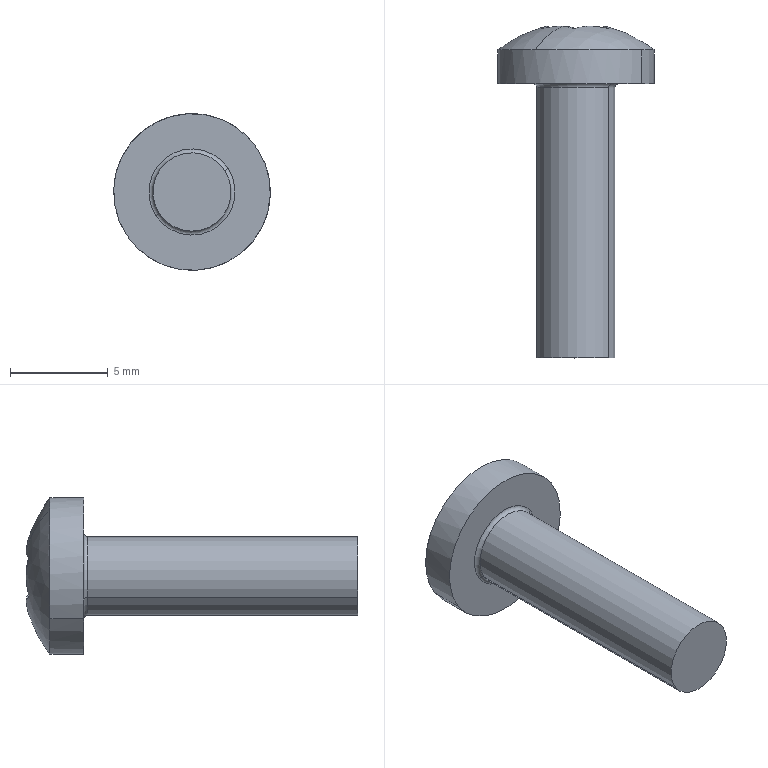Part | SolidWorks | features BaseBody 1 | 1 solid | 23 faces | box 8 x 16.943 x 8 mm | volume 285.559 mm3 | plane 15 | cylinder 4 | sphere 2 | torus 2 | commonest cylinder face diameters 4 x2 8 x2
STEP:
#1=CARTESIAN_POINT('',(202.131,119.073,289.752));
#2=VERTEX_POINT('',#1);
#3=CARTESIAN_POINT('',(203.395,119.073,295.353));
#4=VERTEX_POINT('',#3);
#5=CARTESIAN_POINT('',(205.48,119.073,291.94));
#6=DIRECTION('',(0.,1.,0.));
#7=DIRECTION('',(0.8372,0.,0.5469));
#8=AXIS2_PLACEMENT_3D('',#5,#6,#7);
#9=CIRCLE('',#8,4.);
#10=EDGE_CURVE('',#2,#4,#9,.T.);
#11=ORIENTED_EDGE('',*,*,#10,.T.);
#12=CARTESIAN_POINT('',(204.804,120.281,293.249));
#13=VERTEX_POINT('',#12);
#14=CARTESIAN_POINT('',(205.48,113.95,291.94));
#15=DIRECTION('',(-0.8369,0.02365,-0.5468));
#16=DIRECTION('',(-0.5469,0.,0.8372));
#17=AXIS2_PLACEMENT_3D('',#14,#15,#16);
#18=CIRCLE('',#17,6.5);
#19=EDGE_CURVE('',#4,#13,#18,.T.);
#20=ORIENTED_EDGE('',*,*,#19,.T.);
#21=CARTESIAN_POINT('',(204.702,120.293,293.13));
#22=VERTEX_POINT('',#21);
#23=CARTESIAN_POINT('',(204.443,113.95,292.828));
#24=DIRECTION('',(-0.7597,0.,0.6503));
#25=DIRECTION('',(0.1461,0.9744,0.1706));
#26=AXIS2_PLACEMENT_3D('',#23,#24,#25);
#27=CIRCLE('',#26,6.355);
#28=EDGE_CURVE('',#13,#22,#27,.T.);
#29=ORIENTED_EDGE('',*,*,#28,.T.);
#30=CARTESIAN_POINT('',(203.718,120.143,292.832));
#31=VERTEX_POINT('',#30);
#32=CARTESIAN_POINT('',(205.084,113.95,293.246));
#33=DIRECTION('',(-0.2903,0.,0.9569));
#34=DIRECTION('',(-0.06003,0.998,-0.01821));
#35=AXIS2_PLACEMENT_3D('',#32,#33,#34);
#36=CIRCLE('',#35,6.355);
#37=EDGE_CURVE('',#22,#31,#36,.T.);
#38=ORIENTED_EDGE('',*,*,#37,.T.);
#39=CARTESIAN_POINT('',(204.06,120.293,291.862));
#40=VERTEX_POINT('',#39);
#41=CARTESIAN_POINT('',(204.193,113.95,291.486));
#42=DIRECTION('',(-0.943,0.,-0.3328));
#43=DIRECTION('',(-0.07475,0.9744,0.2118));
#44=AXIS2_PLACEMENT_3D('',#41,#42,#43);
#45=CIRCLE('',#44,6.355);
#46=EDGE_CURVE('',#31,#40,#45,.T.);
#47=ORIENTED_EDGE('',*,*,#46,.T.);
#48=CARTESIAN_POINT('',(203.827,120.143,290.86));
#49=VERTEX_POINT('',#48);
#50=CARTESIAN_POINT('',(204.151,113.95,292.25));
#51=DIRECTION('',(-0.9739,0.,0.227));
#52=DIRECTION('',(-0.01424,0.998,-0.06109));
#53=AXIS2_PLACEMENT_3D('',#50,#51,#52);
#54=CIRCLE('',#53,6.355);
#55=EDGE_CURVE('',#40,#49,#54,.T.);
#56=ORIENTED_EDGE('',*,*,#55,.T.);
#57=CARTESIAN_POINT('',(204.838,120.293,290.671));
#58=VERTEX_POINT('',#57);
#59=CARTESIAN_POINT('',(205.23,113.95,290.598));
#60=DIRECTION('',(-0.1833,0.,-0.9831));
#61=DIRECTION('',(-0.2208,0.9744,0.04117));
#62=AXIS2_PLACEMENT_3D('',#59,#60,#61);
#63=CIRCLE('',#62,6.355);
#64=EDGE_CURVE('',#49,#58,#63,.T.);
#65=ORIENTED_EDGE('',*,*,#64,.T.);
#66=CARTESIAN_POINT('',(205.589,120.143,289.968));
#67=VERTEX_POINT('',#66);
#68=CARTESIAN_POINT('',(204.547,113.95,290.944));
#69=DIRECTION('',(-0.6836,0.,-0.7299));
#70=DIRECTION('',(0.04578,0.998,-0.04288));
#71=AXIS2_PLACEMENT_3D('',#68,#69,#70);
#72=CIRCLE('',#71,6.355);
#73=EDGE_CURVE('',#58,#67,#72,.T.);
#74=ORIENTED_EDGE('',*,*,#73,.T.);
#75=CARTESIAN_POINT('',(206.258,120.293,290.75));
#76=VERTEX_POINT('',#75);
#77=CARTESIAN_POINT('',(206.517,113.95,291.052));
#78=DIRECTION('',(0.7597,0.,-0.6503));
#79=DIRECTION('',(-0.1461,0.9744,-0.1706));
#80=AXIS2_PLACEMENT_3D('',#77,#78,#79);
#81=CIRCLE('',#80,6.355);
#82=EDGE_CURVE('',#67,#76,#81,.T.);
#83=ORIENTED_EDGE('',*,*,#82,.T.);
#84=CARTESIAN_POINT('',(206.407,120.281,290.795));
#85=VERTEX_POINT('',#84);
#86=CARTESIAN_POINT('',(205.876,113.95,290.634));
#87=DIRECTION('',(0.2903,0.,-0.9569));
#88=DIRECTION('',(0.06003,0.998,0.01821));
#89=AXIS2_PLACEMENT_3D('',#86,#87,#88);
#90=CIRCLE('',#89,6.355);
#91=EDGE_CURVE('',#76,#85,#90,.T.);
#92=ORIENTED_EDGE('',*,*,#91,.T.);
#93=CARTESIAN_POINT('',(207.768,119.073,288.659));
#94=VERTEX_POINT('',#93);
#95=CARTESIAN_POINT('',(205.48,113.95,291.94));
#96=DIRECTION('',(-0.8369,0.02365,-0.5468));
#97=DIRECTION('',(-0.5469,0.,0.8372));
#98=AXIS2_PLACEMENT_3D('',#95,#96,#97);
#99=CIRCLE('',#98,6.5);
#100=EDGE_CURVE('',#85,#94,#99,.T.);
#101=ORIENTED_EDGE('',*,*,#100,.T.);
#102=CARTESIAN_POINT('',(205.48,119.073,291.94));
#103=DIRECTION('',(0.,1.,0.));
#104=DIRECTION('',(0.8372,0.,0.5469));
#105=AXIS2_PLACEMENT_3D('',#102,#103,#104);
#106=CIRCLE('',#105,4.);
#107=EDGE_CURVE('',#94,#2,#106,.T.);
#108=ORIENTED_EDGE('',*,*,#107,.T.);
#109=EDGE_LOOP('',(#11,#20,#29,#38,#47,#56,#65,#74,#83,#92,#101,#108));
#110=FACE_OUTER_BOUND('',#109,.T.);
#111=CARTESIAN_POINT('',(205.48,113.95,291.94));
#112=DIRECTION('',(0.8369,-0.02365,0.5468));
#113=DIRECTION('',(0.0198,0.9997,0.01294));
#114=AXIS2_PLACEMENT_3D('',#111,#112,#113);
#115=SPHERICAL_SURFACE('',#114,6.5);
#116=ADVANCED_FACE('',(#110),#115,.T.);
#117=CARTESIAN_POINT('',(202.131,117.35,289.752));
#118=VERTEX_POINT('',#117);
#119=CARTESIAN_POINT('',(208.829,117.35,294.128));
#120=VERTEX_POINT('',#119);
#121=CARTESIAN_POINT('',(205.48,117.35,291.94));
#122=DIRECTION('',(0.,1.,0.));
#123=DIRECTION('',(0.8372,0.,0.5469));
#124=AXIS2_PLACEMENT_3D('',#121,#122,#123);
#125=CIRCLE('',#124,4.);
#126=EDGE_CURVE('',#118,#120,#125,.T.);
#127=ORIENTED_EDGE('',*,*,#126,.T.);
#128=CARTESIAN_POINT('',(208.829,119.073,294.128));
#129=VERTEX_POINT('',#128);
#130=CARTESIAN_POINT('',(208.829,117.35,294.128));
#131=DIRECTION('',(0.,1.,0.));
#132=VECTOR('',#131,1000.);
#133=LINE('',#130,#132);
#134=EDGE_CURVE('',#120,#129,#133,.T.);
#135=ORIENTED_EDGE('',*,*,#134,.T.);
#136=CARTESIAN_POINT('',(205.48,119.073,291.94));
#137=DIRECTION('',(0.,1.,0.));
#138=DIRECTION('',(0.8372,0.,0.5469));
#139=AXIS2_PLACEMENT_3D('',#136,#137,#138);
#140=CIRCLE('',#139,4.);
#141=EDGE_CURVE('',#4,#129,#140,.T.);
#142=ORIENTED_EDGE('',*,*,#141,.F.);
#143=ORIENTED_EDGE('',*,*,#10,.F.);
#144=CARTESIAN_POINT('',(202.131,117.35,289.752));
#145=DIRECTION('',(0.,1.,0.));
#146=VECTOR('',#145,1000.);
#147=LINE('',#144,#146);
#148=EDGE_CURVE('',#118,#2,#147,.T.);
#149=ORIENTED_EDGE('',*,*,#148,.F.);
#150=EDGE_LOOP('',(#127,#135,#142,#143,#149));
#151=FACE_OUTER_BOUND('',#150,.T.);
#152=CARTESIAN_POINT('',(205.48,117.35,291.94));
#153=DIRECTION('',(0.,1.,0.));
#154=DIRECTION('',(-0.8372,0.,-0.5469));
#155=AXIS2_PLACEMENT_3D('',#152,#153,#154);
#156=CYLINDRICAL_SURFACE('',#155,4.);
#157=ADVANCED_FACE('',(#151),#156,.T.);
#158=CARTESIAN_POINT('',(207.154,103.35,293.034));
#159=VERTEX_POINT('',#158);
#160=CARTESIAN_POINT('',(203.806,103.35,290.846));
#161=VERTEX_POINT('',#160);
#162=CARTESIAN_POINT('',(205.48,103.35,291.94));
#163=DIRECTION('',(0.,-1.,0.));
#164=DIRECTION('',(0.8372,0.,0.5469));
#165=AXIS2_PLACEMENT_3D('',#162,#163,#164);
#166=CIRCLE('',#165,2.);
#167=EDGE_CURVE('',#159,#161,#166,.T.);
#168=ORIENTED_EDGE('',*,*,#167,.F.);
#169=CARTESIAN_POINT('',(207.154,117.15,293.034));
#170=VERTEX_POINT('',#169);
#171=CARTESIAN_POINT('',(207.154,103.35,293.034));
#172=DIRECTION('',(0.,1.,0.));
#173=VECTOR('',#172,1000.);
#174=LINE('',#171,#173);
#175=EDGE_CURVE('',#159,#170,#174,.T.);
#176=ORIENTED_EDGE('',*,*,#175,.T.);
#177=CARTESIAN_POINT('',(203.806,117.15,290.846));
#178=VERTEX_POINT('',#177);
#179=CARTESIAN_POINT('',(205.48,117.15,291.94));
#180=DIRECTION('',(0.,-1.,0.));
#181=DIRECTION('',(0.8372,0.,0.5469));
#182=AXIS2_PLACEMENT_3D('',#179,#180,#181);
#183=CIRCLE('',#182,2.);
#184=EDGE_CURVE('',#170,#178,#183,.T.);
#185=ORIENTED_EDGE('',*,*,#184,.T.);
#186=CARTESIAN_POINT('',(203.806,103.35,290.846));
#187=DIRECTION('',(0.,1.,0.));
#188=VECTOR('',#187,1000.);
#189=LINE('',#186,#188);
#190=EDGE_CURVE('',#161,#178,#189,.T.);
#191=ORIENTED_EDGE('',*,*,#190,.F.);
#192=EDGE_LOOP('',(#168,#176,#185,#191));
#193=FACE_OUTER_BOUND('',#192,.T.);
#194=CARTESIAN_POINT('',(205.48,103.35,291.94));
#195=DIRECTION('',(0.,1.,0.));
#196=DIRECTION('',(-0.8372,0.,-0.5469));
#197=AXIS2_PLACEMENT_3D('',#194,#195,#196);
#198=CYLINDRICAL_SURFACE('',#197,2.);
#199=ADVANCED_FACE('',(#193),#198,.T.);
#200=CARTESIAN_POINT('',(207.322,117.35,293.143));
#201=VERTEX_POINT('',#200);
#202=CARTESIAN_POINT('',(203.638,117.35,290.737));
#203=VERTEX_POINT('',#202);
#204=CARTESIAN_POINT('',(205.48,117.35,291.94));
#205=DIRECTION('',(0.,1.,0.));
#206=DIRECTION('',(0.8372,0.,0.5469));
#207=AXIS2_PLACEMENT_3D('',#204,#205,#206);
#208=CIRCLE('',#207,2.2);
#209=EDGE_CURVE('',#201,#203,#208,.T.);
#210=ORIENTED_EDGE('',*,*,#209,.F.);
#211=CARTESIAN_POINT('',(207.322,117.15,293.143));
#212=DIRECTION('',(-0.5469,0.,0.8372));
#213=DIRECTION('',(0.8372,0.,0.5469));
#214=AXIS2_PLACEMENT_3D('',#211,#212,#213);
#215=CIRCLE('',#214,0.2);
#216=EDGE_CURVE('',#201,#170,#215,.T.);
#217=ORIENTED_EDGE('',*,*,#216,.T.);
#218=CARTESIAN_POINT('',(205.48,117.15,291.94));
#219=DIRECTION('',(0.,-1.,0.));
#220=DIRECTION('',(0.8372,0.,0.5469));
#221=AXIS2_PLACEMENT_3D('',#218,#219,#220);
#222=CIRCLE('',#221,2.);
#223=EDGE_CURVE('',#178,#170,#222,.T.);
#224=ORIENTED_EDGE('',*,*,#223,.F.);
#225=CARTESIAN_POINT('',(203.638,117.15,290.737));
#226=DIRECTION('',(0.5469,0.,-0.8372));
#227=DIRECTION('',(-0.8372,0.,-0.5469));
#228=AXIS2_PLACEMENT_3D('',#225,#226,#227);
#229=CIRCLE('',#228,0.2);
#230=EDGE_CURVE('',#203,#178,#229,.T.);
#231=ORIENTED_EDGE('',*,*,#230,.F.);
#232=EDGE_LOOP('',(#210,#217,#224,#231));
#233=FACE_OUTER_BOUND('',#232,.T.);
#234=CARTESIAN_POINT('',(205.48,117.15,291.94));
#235=DIRECTION('',(0.,1.,0.));
#236=DIRECTION('',(-0.8372,0.,-0.5469));
#237=AXIS2_PLACEMENT_3D('',#234,#235,#236);
#238=TOROIDAL_SURFACE('',#237,2.2,0.2);
#239=ADVANCED_FACE('',(#233),#238,.F.);
#240=CARTESIAN_POINT('',(206.9,118.79,292.018));
#241=VERTEX_POINT('',#240);
#242=CARTESIAN_POINT('',(207.133,118.79,293.02));
#243=VERTEX_POINT('',#242);
#244=CARTESIAN_POINT('',(206.9,118.79,292.018));
#245=DIRECTION('',(0.227,0.,0.9739));
#246=VECTOR('',#245,1000.);
#247=LINE('',#244,#246);
#248=EDGE_CURVE('',#241,#243,#247,.T.);
#249=ORIENTED_EDGE('',*,*,#248,.F.);
#250=CARTESIAN_POINT('',(207.242,118.79,291.048));
#251=VERTEX_POINT('',#250);
#252=CARTESIAN_POINT('',(207.242,118.79,291.048));
#253=DIRECTION('',(-0.3328,0.,0.943));
#254=VECTOR('',#253,1000.);
#255=LINE('',#252,#254);
#256=EDGE_CURVE('',#251,#241,#255,.T.);
#257=ORIENTED_EDGE('',*,*,#256,.F.);
#258=CARTESIAN_POINT('',(206.258,118.79,290.75));
#259=VERTEX_POINT('',#258);
#260=CARTESIAN_POINT('',(206.258,118.79,290.75));
#261=DIRECTION('',(0.9569,0.,0.2903));
#262=VECTOR('',#261,1000.);
#263=LINE('',#260,#262);
#264=EDGE_CURVE('',#259,#251,#263,.T.);
#265=ORIENTED_EDGE('',*,*,#264,.F.);
#266=CARTESIAN_POINT('',(205.589,118.79,289.968));
#267=VERTEX_POINT('',#266);
#268=CARTESIAN_POINT('',(205.589,118.79,289.968));
#269=DIRECTION('',(0.6503,0.,0.7597));
#270=VECTOR('',#269,1000.);
#271=LINE('',#268,#270);
#272=EDGE_CURVE('',#267,#259,#271,.T.);
#273=ORIENTED_EDGE('',*,*,#272,.F.);
#274=CARTESIAN_POINT('',(204.838,118.79,290.671));
#275=VERTEX_POINT('',#274);
#276=CARTESIAN_POINT('',(204.838,118.79,290.671));
#277=DIRECTION('',(0.7299,0.,-0.6836));
#278=VECTOR('',#277,1000.);
#279=LINE('',#276,#278);
#280=EDGE_CURVE('',#275,#267,#279,.T.);
#281=ORIENTED_EDGE('',*,*,#280,.F.);
#282=CARTESIAN_POINT('',(203.827,118.79,290.86));
#283=VERTEX_POINT('',#282);
#284=CARTESIAN_POINT('',(203.827,118.79,290.86));
#285=DIRECTION('',(0.9831,0.,-0.1833));
#286=VECTOR('',#285,1000.);
#287=LINE('',#284,#286);
#288=EDGE_CURVE('',#283,#275,#287,.T.);
#289=ORIENTED_EDGE('',*,*,#288,.F.);
#290=CARTESIAN_POINT('',(204.06,118.79,291.862));
#291=VERTEX_POINT('',#290);
#292=CARTESIAN_POINT('',(204.06,118.79,291.862));
#293=DIRECTION('',(-0.227,0.,-0.9739));
#294=VECTOR('',#293,1000.);
#295=LINE('',#292,#294);
#296=EDGE_CURVE('',#291,#283,#295,.T.);
#297=ORIENTED_EDGE('',*,*,#296,.F.);
#298=CARTESIAN_POINT('',(203.718,118.79,292.832));
#299=VERTEX_POINT('',#298);
#300=CARTESIAN_POINT('',(203.718,118.79,292.832));
#301=DIRECTION('',(0.3328,0.,-0.943));
#302=VECTOR('',#301,1000.);
#303=LINE('',#300,#302);
#304=EDGE_CURVE('',#299,#291,#303,.T.);
#305=ORIENTED_EDGE('',*,*,#304,.F.);
#306=CARTESIAN_POINT('',(204.702,118.79,293.13));
#307=VERTEX_POINT('',#306);
#308=CARTESIAN_POINT('',(204.702,118.79,293.13));
#309=DIRECTION('',(-0.9569,0.,-0.2903));
#310=VECTOR('',#309,1000.);
#311=LINE('',#308,#310);
#312=EDGE_CURVE('',#307,#299,#311,.T.);
#313=ORIENTED_EDGE('',*,*,#312,.F.);
#314=CARTESIAN_POINT('',(205.371,118.79,293.912));
#315=VERTEX_POINT('',#314);
#316=CARTESIAN_POINT('',(205.371,118.79,293.912));
#317=DIRECTION('',(-0.6503,0.,-0.7597));
#318=VECTOR('',#317,1000.);
#319=LINE('',#316,#318);
#320=EDGE_CURVE('',#315,#307,#319,.T.);
#321=ORIENTED_EDGE('',*,*,#320,.F.);
#322=CARTESIAN_POINT('',(206.122,118.79,293.209));
#323=VERTEX_POINT('',#322);
#324=CARTESIAN_POINT('',(206.122,118.79,293.209));
#325=DIRECTION('',(-0.7299,0.,0.6836));
#326=VECTOR('',#325,1000.);
#327=LINE('',#324,#326);
#328=EDGE_CURVE('',#323,#315,#327,.T.);
#329=ORIENTED_EDGE('',*,*,#328,.F.);
#330=CARTESIAN_POINT('',(207.133,118.79,293.02));
#331=DIRECTION('',(-0.9831,0.,0.1833));
#332=VECTOR('',#331,1000.);
#333=LINE('',#330,#332);
#334=EDGE_CURVE('',#243,#323,#333,.T.);
#335=ORIENTED_EDGE('',*,*,#334,.F.);
#336=EDGE_LOOP('',(#249,#257,#265,#273,#281,#289,#297,#305,#313,#321,#329,#335));
#337=FACE_OUTER_BOUND('',#336,.T.);
#338=CARTESIAN_POINT('',(206.513,118.79,290.359));
#339=DIRECTION('',(0.,1.,0.));
#340=DIRECTION('',(1.,0.,0.));
#341=AXIS2_PLACEMENT_3D('',#338,#339,#340);
#342=PLANE('',#341);
#343=ADVANCED_FACE('',(#337),#342,.T.);
#344=CARTESIAN_POINT('',(207.133,120.143,293.02));
#345=VERTEX_POINT('',#344);
#346=CARTESIAN_POINT('',(207.133,118.79,293.02));
#347=DIRECTION('',(0.,1.,0.));
#348=VECTOR('',#347,1000.);
#349=LINE('',#346,#348);
#350=EDGE_CURVE('',#243,#345,#349,.T.);
#351=ORIENTED_EDGE('',*,*,#350,.F.);
#352=ORIENTED_EDGE('',*,*,#334,.T.);
#353=CARTESIAN_POINT('',(206.122,120.293,293.209));
#354=VERTEX_POINT('',#353);
#355=CARTESIAN_POINT('',(206.122,120.293,293.209));
#356=DIRECTION('',(0.,-1.,0.));
#357=VECTOR('',#356,1000.);
#358=LINE('',#355,#357);
#359=EDGE_CURVE('',#354,#323,#358,.T.);
#360=ORIENTED_EDGE('',*,*,#359,.F.);
#361=CARTESIAN_POINT('',(205.73,113.95,293.282));
#362=DIRECTION('',(0.1833,0.,0.9831));
#363=DIRECTION('',(0.2208,0.9744,-0.04117));
#364=AXIS2_PLACEMENT_3D('',#361,#362,#363);
#365=CIRCLE('',#364,6.355);
#366=EDGE_CURVE('',#345,#354,#365,.T.);
#367=ORIENTED_EDGE('',*,*,#366,.F.);
#368=EDGE_LOOP('',(#351,#352,#360,#367));
#369=FACE_OUTER_BOUND('',#368,.T.);
#370=CARTESIAN_POINT('',(206.122,118.79,293.209));
#371=DIRECTION('',(-0.1833,0.,-0.9831));
#372=DIRECTION('',(-0.9831,0.,0.1833));
#373=AXIS2_PLACEMENT_3D('',#370,#371,#372);
#374=PLANE('',#373);
#375=ADVANCED_FACE('',(#369),#374,.T.);
#376=ORIENTED_EDGE('',*,*,#359,.T.);
#377=ORIENTED_EDGE('',*,*,#328,.T.);
#378=CARTESIAN_POINT('',(205.371,120.143,293.912));
#379=VERTEX_POINT('',#378);
#380=CARTESIAN_POINT('',(205.371,120.143,293.912));
#381=DIRECTION('',(0.,-1.,0.));
#382=VECTOR('',#381,1000.);
#383=LINE('',#380,#382);
#384=EDGE_CURVE('',#379,#315,#383,.T.);
#385=ORIENTED_EDGE('',*,*,#384,.F.);
#386=CARTESIAN_POINT('',(206.413,113.95,292.936));
#387=DIRECTION('',(0.6836,0.,0.7299));
#388=DIRECTION('',(-0.04578,0.998,0.04288));
#389=AXIS2_PLACEMENT_3D('',#386,#387,#388);
#390=CIRCLE('',#389,6.355);
#391=EDGE_CURVE('',#354,#379,#390,.T.);
#392=ORIENTED_EDGE('',*,*,#391,.F.);
#393=EDGE_LOOP('',(#376,#377,#385,#392));
#394=FACE_OUTER_BOUND('',#393,.T.);
#395=CARTESIAN_POINT('',(205.371,118.79,293.912));
#396=DIRECTION('',(-0.6836,0.,-0.7299));
#397=DIRECTION('',(-0.7299,0.,0.6836));
#398=AXIS2_PLACEMENT_3D('',#395,#396,#397);
#399=PLANE('',#398);
#400=ADVANCED_FACE('',(#394),#399,.T.);
#401=ORIENTED_EDGE('',*,*,#384,.T.);
#402=ORIENTED_EDGE('',*,*,#320,.T.);
#403=CARTESIAN_POINT('',(204.702,120.293,293.13));
#404=DIRECTION('',(0.,-1.,0.));
#405=VECTOR('',#404,1000.);
#406=LINE('',#403,#405);
#407=EDGE_CURVE('',#22,#307,#406,.T.);
#408=ORIENTED_EDGE('',*,*,#407,.F.);
#409=ORIENTED_EDGE('',*,*,#28,.F.);
#410=CARTESIAN_POINT('',(204.443,113.95,292.828));
#411=DIRECTION('',(-0.7597,0.,0.6503));
#412=DIRECTION('',(0.1461,0.9744,0.1706));
#413=AXIS2_PLACEMENT_3D('',#410,#411,#412);
#414=CIRCLE('',#413,6.355);
#415=EDGE_CURVE('',#379,#13,#414,.T.);
#416=ORIENTED_EDGE('',*,*,#415,.F.);
#417=EDGE_LOOP('',(#401,#402,#408,#409,#416));
#418=FACE_OUTER_BOUND('',#417,.T.);
#419=CARTESIAN_POINT('',(204.702,118.79,293.13));
#420=DIRECTION('',(0.7597,0.,-0.6503));
#421=DIRECTION('',(0.,-1.,0.));
#422=AXIS2_PLACEMENT_3D('',#419,#420,#421);
#423=PLANE('',#422);
#424=ADVANCED_FACE('',(#418),#423,.T.);
#425=ORIENTED_EDGE('',*,*,#407,.T.);
#426=ORIENTED_EDGE('',*,*,#312,.T.);
#427=CARTESIAN_POINT('',(203.718,120.143,292.832));
#428=DIRECTION('',(0.,-1.,0.));
#429=VECTOR('',#428,1000.);
#430=LINE('',#427,#429);
#431=EDGE_CURVE('',#31,#299,#430,.T.);
#432=ORIENTED_EDGE('',*,*,#431,.F.);
#433=ORIENTED_EDGE('',*,*,#37,.F.);
#434=EDGE_LOOP('',(#425,#426,#432,#433));
#435=FACE_OUTER_BOUND('',#434,.T.);
#436=CARTESIAN_POINT('',(203.718,118.79,292.832));
#437=DIRECTION('',(0.2903,0.,-0.9569));
#438=DIRECTION('',(0.,-1.,0.));
#439=AXIS2_PLACEMENT_3D('',#436,#437,#438);
#440=PLANE('',#439);
#441=ADVANCED_FACE('',(#435),#440,.T.);
#442=ORIENTED_EDGE('',*,*,#431,.T.);
#443=ORIENTED_EDGE('',*,*,#304,.T.);
#444=CARTESIAN_POINT('',(204.06,120.293,291.862));
#445=DIRECTION('',(0.,-1.,0.));
#446=VECTOR('',#445,1000.);
#447=LINE('',#444,#446);
#448=EDGE_CURVE('',#40,#291,#447,.T.);
#449=ORIENTED_EDGE('',*,*,#448,.F.);
#450=ORIENTED_EDGE('',*,*,#46,.F.);
#451=EDGE_LOOP('',(#442,#443,#449,#450));
#452=FACE_OUTER_BOUND('',#451,.T.);
#453=CARTESIAN_POINT('',(204.06,118.79,291.862));
#454=DIRECTION('',(0.943,0.,0.3328));
#455=DIRECTION('',(0.,-1.,0.));
#456=AXIS2_PLACEMENT_3D('',#453,#454,#455);
#457=PLANE('',#456);
#458=ADVANCED_FACE('',(#452),#457,.T.);
#459=ORIENTED_EDGE('',*,*,#448,.T.);
#460=ORIENTED_EDGE('',*,*,#296,.T.);
#461=CARTESIAN_POINT('',(203.827,120.143,290.86));
#462=DIRECTION('',(0.,-1.,0.));
#463=VECTOR('',#462,1000.);
#464=LINE('',#461,#463);
#465=EDGE_CURVE('',#49,#283,#464,.T.);
#466=ORIENTED_EDGE('',*,*,#465,.F.);
#467=ORIENTED_EDGE('',*,*,#55,.F.);
#468=EDGE_LOOP('',(#459,#460,#466,#467));
#469=FACE_OUTER_BOUND('',#468,.T.);
#470=CARTESIAN_POINT('',(203.827,118.79,290.86));
#471=DIRECTION('',(0.9739,0.,-0.227));
#472=DIRECTION('',(0.,-1.,0.));
#473=AXIS2_PLACEMENT_3D('',#470,#471,#472);
#474=PLANE('',#473);
#475=ADVANCED_FACE('',(#469),#474,.T.);
#476=ORIENTED_EDGE('',*,*,#465,.T.);
#477=ORIENTED_EDGE('',*,*,#288,.T.);
#478=CARTESIAN_POINT('',(204.838,120.293,290.671));
#479=DIRECTION('',(0.,-1.,0.));
#480=VECTOR('',#479,1000.);
#481=LINE('',#478,#480);
#482=EDGE_CURVE('',#58,#275,#481,.T.);
#483=ORIENTED_EDGE('',*,*,#482,.F.);
#484=ORIENTED_EDGE('',*,*,#64,.F.);
#485=EDGE_LOOP('',(#476,#477,#483,#484));
#486=FACE_OUTER_BOUND('',#485,.T.);
#487=CARTESIAN_POINT('',(204.838,118.79,290.671));
#488=DIRECTION('',(0.1833,0.,0.9831));
#489=DIRECTION('',(0.,-1.,0.));
#490=AXIS2_PLACEMENT_3D('',#487,#488,#489);
#491=PLANE('',#490);
#492=ADVANCED_FACE('',(#486),#491,.T.);
#493=ORIENTED_EDGE('',*,*,#482,.T.);
#494=ORIENTED_EDGE('',*,*,#280,.T.);
#495=CARTESIAN_POINT('',(205.589,120.143,289.968));
#496=DIRECTION('',(0.,-1.,0.));
#497=VECTOR('',#496,1000.);
#498=LINE('',#495,#497);
#499=EDGE_CURVE('',#67,#267,#498,.T.);
#500=ORIENTED_EDGE('',*,*,#499,.F.);
#501=ORIENTED_EDGE('',*,*,#73,.F.);
#502=EDGE_LOOP('',(#493,#494,#500,#501));
#503=FACE_OUTER_BOUND('',#502,.T.);
#504=CARTESIAN_POINT('',(205.589,118.79,289.968));
#505=DIRECTION('',(0.6836,0.,0.7299));
#506=DIRECTION('',(0.,-1.,0.));
#507=AXIS2_PLACEMENT_3D('',#504,#505,#506);
#508=PLANE('',#507);
#509=ADVANCED_FACE('',(#503),#508,.T.);
#510=ORIENTED_EDGE('',*,*,#499,.T.);
#511=ORIENTED_EDGE('',*,*,#272,.T.);
#512=CARTESIAN_POINT('',(206.258,120.293,290.75));
#513=DIRECTION('',(0.,-1.,0.));
#514=VECTOR('',#513,1000.);
#515=LINE('',#512,#514);
#516=EDGE_CURVE('',#76,#259,#515,.T.);
#517=ORIENTED_EDGE('',*,*,#516,.F.);
#518=ORIENTED_EDGE('',*,*,#82,.F.);
#519=EDGE_LOOP('',(#510,#511,#517,#518));
#520=FACE_OUTER_BOUND('',#519,.T.);
#521=CARTESIAN_POINT('',(206.258,118.79,290.75));
#522=DIRECTION('',(-0.7597,0.,0.6503));
#523=DIRECTION('',(0.,1.,0.));
#524=AXIS2_PLACEMENT_3D('',#521,#522,#523);
#525=PLANE('',#524);
#526=ADVANCED_FACE('',(#520),#525,.T.);
#527=ORIENTED_EDGE('',*,*,#516,.T.);
#528=ORIENTED_EDGE('',*,*,#264,.T.);
#529=CARTESIAN_POINT('',(207.242,120.143,291.048));
#530=VERTEX_POINT('',#529);
#531=CARTESIAN_POINT('',(207.242,120.143,291.048));
#532=DIRECTION('',(0.,-1.,0.));
#533=VECTOR('',#532,1000.);
#534=LINE('',#531,#533);
#535=EDGE_CURVE('',#530,#251,#534,.T.);
#536=ORIENTED_EDGE('',*,*,#535,.F.);
#537=CARTESIAN_POINT('',(205.876,113.95,290.634));
#538=DIRECTION('',(0.2903,0.,-0.9569));
#539=DIRECTION('',(0.06003,0.998,0.01821));
#540=AXIS2_PLACEMENT_3D('',#537,#538,#539);
#541=CIRCLE('',#540,6.355);
#542=EDGE_CURVE('',#85,#530,#541,.T.);
#543=ORIENTED_EDGE('',*,*,#542,.F.);
#544=ORIENTED_EDGE('',*,*,#91,.F.);
#545=EDGE_LOOP('',(#527,#528,#536,#543,#544));
#546=FACE_OUTER_BOUND('',#545,.T.);
#547=CARTESIAN_POINT('',(207.242,118.79,291.048));
#548=DIRECTION('',(-0.2903,0.,0.9569));
#549=DIRECTION('',(0.,1.,0.));
#550=AXIS2_PLACEMENT_3D('',#547,#548,#549);
#551=PLANE('',#550);
#552=ADVANCED_FACE('',(#546),#551,.T.);
#553=ORIENTED_EDGE('',*,*,#535,.T.);
#554=ORIENTED_EDGE('',*,*,#256,.T.);
#555=CARTESIAN_POINT('',(206.9,120.293,292.018));
#556=VERTEX_POINT('',#555);
#557=CARTESIAN_POINT('',(206.9,120.293,292.018));
#558=DIRECTION('',(0.,-1.,0.));
#559=VECTOR('',#558,1000.);
#560=LINE('',#557,#559);
#561=EDGE_CURVE('',#556,#241,#560,.T.);
#562=ORIENTED_EDGE('',*,*,#561,.F.);
#563=CARTESIAN_POINT('',(206.767,113.95,292.394));
#564=DIRECTION('',(0.943,0.,0.3328));
#565=DIRECTION('',(0.07475,0.9744,-0.2118));
#566=AXIS2_PLACEMENT_3D('',#563,#564,#565);
#567=CIRCLE('',#566,6.355);
#568=EDGE_CURVE('',#530,#556,#567,.T.);
#569=ORIENTED_EDGE('',*,*,#568,.F.);
#570=EDGE_LOOP('',(#553,#554,#562,#569));
#571=FACE_OUTER_BOUND('',#570,.T.);
#572=CARTESIAN_POINT('',(206.9,118.79,292.018));
#573=DIRECTION('',(-0.943,0.,-0.3328));
#574=DIRECTION('',(-0.3328,0.,0.943));
#575=AXIS2_PLACEMENT_3D('',#572,#573,#574);
#576=PLANE('',#575);
#577=ADVANCED_FACE('',(#571),#576,.T.);
#578=ORIENTED_EDGE('',*,*,#561,.T.);
#579=ORIENTED_EDGE('',*,*,#248,.T.);
#580=ORIENTED_EDGE('',*,*,#350,.T.);
#581=CARTESIAN_POINT('',(206.809,113.95,291.63));
#582=DIRECTION('',(0.9739,0.,-0.227));
#583=DIRECTION('',(0.01424,0.998,0.06109));
#584=AXIS2_PLACEMENT_3D('',#581,#582,#583);
#585=CIRCLE('',#584,6.355);
#586=EDGE_CURVE('',#556,#345,#585,.T.);
#587=ORIENTED_EDGE('',*,*,#586,.F.);
#588=EDGE_LOOP('',(#578,#579,#580,#587));
#589=FACE_OUTER_BOUND('',#588,.T.);
#590=CARTESIAN_POINT('',(207.133,118.79,293.02));
#591=DIRECTION('',(-0.9739,0.,0.227));
#592=DIRECTION('',(0.,1.,0.));
#593=AXIS2_PLACEMENT_3D('',#590,#591,#592);
#594=PLANE('',#593);
#595=ADVANCED_FACE('',(#589),#594,.T.);
#596=ORIENTED_EDGE('',*,*,#216,.F.);
#597=CARTESIAN_POINT('',(205.48,117.35,291.94));
#598=DIRECTION('',(0.,1.,0.));
#599=DIRECTION('',(0.8372,0.,0.5469));
#600=AXIS2_PLACEMENT_3D('',#597,#598,#599);
#601=CIRCLE('',#600,2.2);
#602=EDGE_CURVE('',#203,#201,#601,.T.);
#603=ORIENTED_EDGE('',*,*,#602,.F.);
#604=ORIENTED_EDGE('',*,*,#230,.T.);
#605=ORIENTED_EDGE('',*,*,#184,.F.);
#606=EDGE_LOOP('',(#596,#603,#604,#605));
#607=FACE_OUTER_BOUND('',#606,.T.);
#608=CARTESIAN_POINT('',(205.48,117.15,291.94));
#609=DIRECTION('',(0.,1.,0.));
#610=DIRECTION('',(-0.8372,0.,-0.5469));
#611=AXIS2_PLACEMENT_3D('',#608,#609,#610);
#612=TOROIDAL_SURFACE('',#611,2.2,0.2);
#613=ADVANCED_FACE('',(#607),#612,.F.);
#614=ORIENTED_EDGE('',*,*,#175,.F.);
#615=CARTESIAN_POINT('',(205.48,103.35,291.94));
#616=DIRECTION('',(0.,-1.,0.));
#617=DIRECTION('',(0.8372,0.,0.5469));
#618=AXIS2_PLACEMENT_3D('',#615,#616,#617);
#619=CIRCLE('',#618,2.);
#620=EDGE_CURVE('',#161,#159,#619,.T.);
#621=ORIENTED_EDGE('',*,*,#620,.F.);
#622=ORIENTED_EDGE('',*,*,#190,.T.);
#623=ORIENTED_EDGE('',*,*,#223,.T.);
#624=EDGE_LOOP('',(#614,#621,#622,#623));
#625=FACE_OUTER_BOUND('',#624,.T.);
#626=CARTESIAN_POINT('',(205.48,103.35,291.94));
#627=DIRECTION('',(0.,1.,0.));
#628=DIRECTION('',(-0.8372,0.,-0.5469));
#629=AXIS2_PLACEMENT_3D('',#626,#627,#628);
#630=CYLINDRICAL_SURFACE('',#629,2.);
#631=ADVANCED_FACE('',(#625),#630,.T.);
#632=ORIENTED_EDGE('',*,*,#602,.T.);
#633=ORIENTED_EDGE('',*,*,#209,.T.);
#634=EDGE_LOOP('',(#632,#633));
#635=FACE_BOUND('',#634,.T.);
#636=ORIENTED_EDGE('',*,*,#126,.F.);
#637=CARTESIAN_POINT('',(205.48,117.35,291.94));
#638=DIRECTION('',(0.,1.,0.));
#639=DIRECTION('',(0.8372,0.,0.5469));
#640=AXIS2_PLACEMENT_3D('',#637,#638,#639);
#641=CIRCLE('',#640,4.);
#642=EDGE_CURVE('',#120,#118,#641,.T.);
#643=ORIENTED_EDGE('',*,*,#642,.F.);
#644=EDGE_LOOP('',(#636,#643));
#645=FACE_OUTER_BOUND('',#644,.T.);
#646=CARTESIAN_POINT('',(206.574,117.35,290.266));
#647=DIRECTION('',(0.,-1.,0.));
#648=DIRECTION('',(0.,0.,-1.));
#649=AXIS2_PLACEMENT_3D('',#646,#647,#648);
#650=PLANE('',#649);
#651=ADVANCED_FACE('',(#635,#645),#650,.T.);
#652=ORIENTED_EDGE('',*,*,#134,.F.);
#653=ORIENTED_EDGE('',*,*,#642,.T.);
#654=ORIENTED_EDGE('',*,*,#148,.T.);
#655=ORIENTED_EDGE('',*,*,#107,.F.);
#656=CARTESIAN_POINT('',(205.48,119.073,291.94));
#657=DIRECTION('',(0.,1.,0.));
#658=DIRECTION('',(0.8372,0.,0.5469));
#659=AXIS2_PLACEMENT_3D('',#656,#657,#658);
#660=CIRCLE('',#659,4.);
#661=EDGE_CURVE('',#129,#94,#660,.T.);
#662=ORIENTED_EDGE('',*,*,#661,.F.);
#663=EDGE_LOOP('',(#652,#653,#654,#655,#662));
#664=FACE_OUTER_BOUND('',#663,.T.);
#665=CARTESIAN_POINT('',(205.48,117.35,291.94));
#666=DIRECTION('',(0.,1.,0.));
#667=DIRECTION('',(-0.8372,0.,-0.5469));
#668=AXIS2_PLACEMENT_3D('',#665,#666,#667);
#669=CYLINDRICAL_SURFACE('',#668,4.);
#670=ADVANCED_FACE('',(#664),#669,.T.);
#671=ORIENTED_EDGE('',*,*,#19,.F.);
#672=ORIENTED_EDGE('',*,*,#141,.T.);
#673=ORIENTED_EDGE('',*,*,#661,.T.);
#674=ORIENTED_EDGE('',*,*,#100,.F.);
#675=ORIENTED_EDGE('',*,*,#542,.T.);
#676=ORIENTED_EDGE('',*,*,#568,.T.);
#677=ORIENTED_EDGE('',*,*,#586,.T.);
#678=ORIENTED_EDGE('',*,*,#366,.T.);
#679=ORIENTED_EDGE('',*,*,#391,.T.);
#680=ORIENTED_EDGE('',*,*,#415,.T.);
#681=EDGE_LOOP('',(#671,#672,#673,#674,#675,#676,#677,#678,#679,#680));
#682=FACE_OUTER_BOUND('',#681,.T.);
#683=CARTESIAN_POINT('',(205.48,113.95,291.94));
#684=DIRECTION('',(0.8369,-0.02365,0.5468));
#685=DIRECTION('',(0.0198,0.9997,0.01294));
#686=AXIS2_PLACEMENT_3D('',#683,#684,#685);
#687=SPHERICAL_SURFACE('',#686,6.5);
#688=ADVANCED_FACE('',(#682),#687,.T.);
#689=ORIENTED_EDGE('',*,*,#620,.T.);
#690=ORIENTED_EDGE('',*,*,#167,.T.);
#691=EDGE_LOOP('',(#689,#690));
#692=FACE_OUTER_BOUND('',#691,.T.);
#693=CARTESIAN_POINT('',(205.48,103.35,291.94));
#694=DIRECTION('',(0.,-1.,0.));
#695=DIRECTION('',(0.,0.,-1.));
#696=AXIS2_PLACEMENT_3D('',#693,#694,#695);
#697=PLANE('',#696);
#698=ADVANCED_FACE('',(#692),#697,.T.);
#699=CLOSED_SHELL('',(#116,#157,#199,#239,#343,#375,#400,#424,#441,#458,#475,#492,#509,#526,#552,#577,#595,#613,#631,#651,#670,#688,#698));
#700=MANIFOLD_SOLID_BREP('',#699);
#701=CARTESIAN_POINT('',(0.,0.,0.));
#702=DIRECTION('',(0.,0.,1.));
#703=DIRECTION('',(1.,0.,0.));
#704=AXIS2_PLACEMENT_3D('',#701,#702,#703);
#705=(LENGTH_UNIT()NAMED_UNIT(*)SI_UNIT(.MILLI.,.METRE.));
#706=UNCERTAINTY_MEASURE_WITH_UNIT(LENGTH_MEASURE(0.00001),#705,'','');
#707=(NAMED_UNIT(*)PLANE_ANGLE_UNIT()SI_UNIT($,.RADIAN.));
#708=(NAMED_UNIT(*)SI_UNIT($,.STERADIAN.)SOLID_ANGLE_UNIT());
#709=(GEOMETRIC_REPRESENTATION_CONTEXT(3)GLOBAL_UNCERTAINTY_ASSIGNED_CONTEXT((#706))GLOBAL_UNIT_ASSIGNED_CONTEXT((#705,#707,#708))REPRESENTATION_CONTEXT('',''));
#710=ADVANCED_BREP_SHAPE_REPRESENTATION('',(#700,#704),#709);